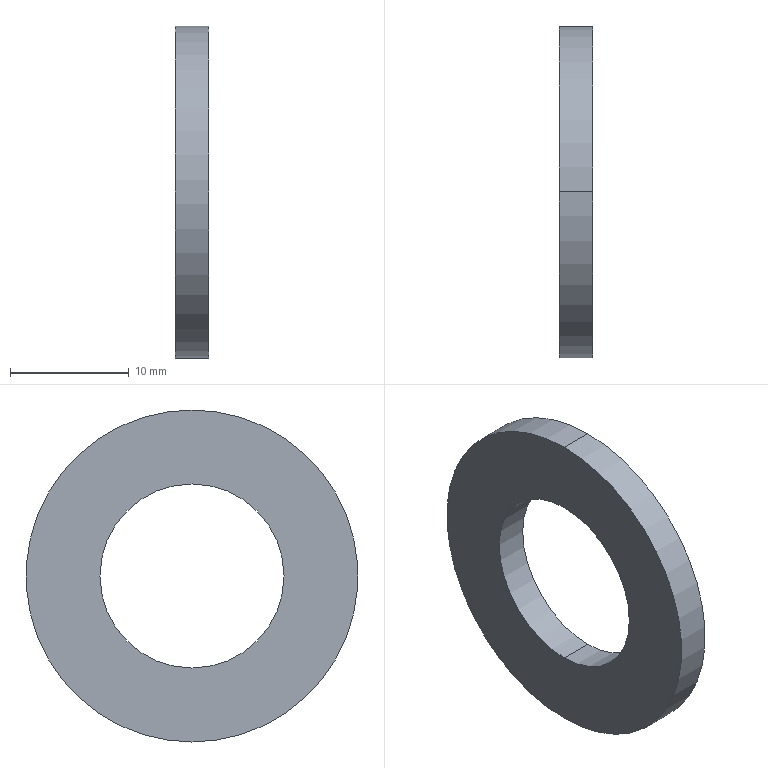Part | STEP file | flat washer narrow_am_B18.22M - Plain washer, 14 mm, narrow | 1 solid | 6 faces | box 2.8 x 28 x 28 mm | volume 1194 mm3 | cylinder 4 | plane 2 | commonest cylinder face diameters 15.52 x2 28 x2
STEP:
#1=CARTESIAN_POINT('',(0.,0.,0.));
#2=DIRECTION('',(0.,0.,1.));
#3=DIRECTION('',(1.,0.,0.));
#4=AXIS2_PLACEMENT_3D('',#1,#2,#3);
#5=CARTESIAN_POINT('',(0.,0.,14.));
#6=VERTEX_POINT('',#5);
#7=CARTESIAN_POINT('',(0.,0.,-14.));
#8=VERTEX_POINT('',#7);
#9=CARTESIAN_POINT('',(0.,0.,0.));
#10=DIRECTION('',(-1.,0.,0.));
#11=DIRECTION('',(0.,0.,1.));
#12=AXIS2_PLACEMENT_3D('',#9,#10,#11);
#13=CIRCLE('',#12,14.);
#14=CARTESIAN_POINT('',(-34.925,0.,0.));
#15=DIRECTION('',(-1.,0.,0.));
#16=DIRECTION('',(0.,0.,1.));
#17=AXIS2_PLACEMENT_3D('',#14,#15,#16);
#18=CYLINDRICAL_SURFACE('',#17,14.);
#19=CARTESIAN_POINT('',(0.,-34.925));
#20=DIRECTION('',(1.,0.));
#21=VECTOR('',#20,1.);
#22=LINE('',#19,#21);
#23=(GEOMETRIC_REPRESENTATION_CONTEXT(2)PARAMETRIC_REPRESENTATION_CONTEXT()REPRESENTATION_CONTEXT('',''));
#24=DEFINITIONAL_REPRESENTATION('',(#22),#23);
#25=PCURVE('',#18,#24);
#26=CARTESIAN_POINT('',(0.,7.76,0.));
#27=DIRECTION('',(-1.,0.,0.));
#28=DIRECTION('',(0.,0.,1.));
#29=AXIS2_PLACEMENT_3D('',#26,#27,#28);
#30=PLANE('',#29);
#31=CARTESIAN_POINT('',(0.,-7.76));
#32=DIRECTION('',(1.,0.));
#33=AXIS2_PLACEMENT_2D('',#31,#32);
#34=CIRCLE('',#33,14.);
#35=(GEOMETRIC_REPRESENTATION_CONTEXT(2)PARAMETRIC_REPRESENTATION_CONTEXT()REPRESENTATION_CONTEXT('',''));
#36=DEFINITIONAL_REPRESENTATION('',(#34),#35);
#37=PCURVE('',#30,#36);
#38=SURFACE_CURVE('',#13,(#25,#37),.PCURVE_S1.);
#39=EDGE_CURVE('',#6,#8,#38,.T.);
#40=ORIENTED_EDGE('',*,*,#39,.T.);
#41=CARTESIAN_POINT('',(-2.8,0.,-14.));
#42=VERTEX_POINT('',#41);
#43=CARTESIAN_POINT('',(-34.925,0.,-14.));
#44=DIRECTION('',(-1.,0.,0.));
#45=VECTOR('',#44,1.);
#46=LINE('',#43,#45);
#47=CARTESIAN_POINT('',(3.142,0.));
#48=DIRECTION('',(0.,1.));
#49=VECTOR('',#48,1.);
#50=LINE('',#47,#49);
#51=(GEOMETRIC_REPRESENTATION_CONTEXT(2)PARAMETRIC_REPRESENTATION_CONTEXT()REPRESENTATION_CONTEXT('',''));
#52=DEFINITIONAL_REPRESENTATION('',(#50),#51);
#53=PCURVE('',#18,#52);
#54=CARTESIAN_POINT('',(-34.925,0.,0.));
#55=DIRECTION('',(-1.,0.,0.));
#56=DIRECTION('',(0.,0.,1.));
#57=AXIS2_PLACEMENT_3D('',#54,#55,#56);
#58=CYLINDRICAL_SURFACE('',#57,14.);
#59=CARTESIAN_POINT('',(3.142,0.));
#60=DIRECTION('',(0.,1.));
#61=VECTOR('',#60,1.);
#62=LINE('',#59,#61);
#63=(GEOMETRIC_REPRESENTATION_CONTEXT(2)PARAMETRIC_REPRESENTATION_CONTEXT()REPRESENTATION_CONTEXT('',''));
#64=DEFINITIONAL_REPRESENTATION('',(#62),#63);
#65=PCURVE('',#58,#64);
#66=SURFACE_CURVE('',#46,(#53,#65),.PCURVE_S1.);
#67=EDGE_CURVE('',#8,#42,#66,.T.);
#68=ORIENTED_EDGE('',*,*,#67,.T.);
#69=CARTESIAN_POINT('',(-2.8,0.,14.));
#70=VERTEX_POINT('',#69);
#71=CARTESIAN_POINT('',(-2.8,0.,0.));
#72=DIRECTION('',(-1.,0.,0.));
#73=DIRECTION('',(0.,0.,1.));
#74=AXIS2_PLACEMENT_3D('',#71,#72,#73);
#75=CIRCLE('',#74,14.);
#76=CARTESIAN_POINT('',(0.,-32.125));
#77=DIRECTION('',(1.,0.));
#78=VECTOR('',#77,1.);
#79=LINE('',#76,#78);
#80=(GEOMETRIC_REPRESENTATION_CONTEXT(2)PARAMETRIC_REPRESENTATION_CONTEXT()REPRESENTATION_CONTEXT('',''));
#81=DEFINITIONAL_REPRESENTATION('',(#79),#80);
#82=PCURVE('',#18,#81);
#83=CARTESIAN_POINT('',(-2.8,14.,0.));
#84=DIRECTION('',(1.,0.,0.));
#85=DIRECTION('',(0.,0.,-1.));
#86=AXIS2_PLACEMENT_3D('',#83,#84,#85);
#87=PLANE('',#86);
#88=CARTESIAN_POINT('',(-14.,-14.));
#89=CARTESIAN_POINT('',(-14.,10.249));
#90=CARTESIAN_POINT('',(7.,-1.876));
#91=CARTESIAN_POINT('',(28.,-14.));
#92=CARTESIAN_POINT('',(7.,-26.124));
#93=CARTESIAN_POINT('',(-14.,-38.249));
#94=CARTESIAN_POINT('',(-14.,-14.));
#95=(BOUNDED_CURVE()B_SPLINE_CURVE(2,(#88,#89,#90,#91,#92,#93,#94),.UNSPECIFIED.,.T.,.F.)B_SPLINE_CURVE_WITH_KNOTS((1,2,2,2,2,1),(-2.094,0.,2.094,4.189,6.283,8.378),.UNSPECIFIED.)CURVE()GEOMETRIC_REPRESENTATION_ITEM()RATIONAL_B_SPLINE_CURVE((1.,0.5,1.,0.5,1.,0.5,1.))REPRESENTATION_ITEM(''));
#96=(GEOMETRIC_REPRESENTATION_CONTEXT(2)PARAMETRIC_REPRESENTATION_CONTEXT()REPRESENTATION_CONTEXT('',''));
#97=DEFINITIONAL_REPRESENTATION('',(#95),#96);
#98=PCURVE('',#87,#97);
#99=SURFACE_CURVE('',#75,(#82,#98),.PCURVE_S1.);
#100=EDGE_CURVE('',#70,#42,#99,.T.);
#101=ORIENTED_EDGE('',*,*,#100,.F.);
#102=CARTESIAN_POINT('',(-34.925,0.,14.));
#103=DIRECTION('',(-1.,0.,0.));
#104=VECTOR('',#103,1.);
#105=LINE('',#102,#104);
#106=CARTESIAN_POINT('',(0.,0.));
#107=DIRECTION('',(0.,1.));
#108=VECTOR('',#107,1.);
#109=LINE('',#106,#108);
#110=(GEOMETRIC_REPRESENTATION_CONTEXT(2)PARAMETRIC_REPRESENTATION_CONTEXT()REPRESENTATION_CONTEXT('',''));
#111=DEFINITIONAL_REPRESENTATION('',(#109),#110);
#112=PCURVE('',#18,#111);
#113=CARTESIAN_POINT('',(6.283,0.));
#114=DIRECTION('',(0.,1.));
#115=VECTOR('',#114,1.);
#116=LINE('',#113,#115);
#117=(GEOMETRIC_REPRESENTATION_CONTEXT(2)PARAMETRIC_REPRESENTATION_CONTEXT()REPRESENTATION_CONTEXT('',''));
#118=DEFINITIONAL_REPRESENTATION('',(#116),#117);
#119=PCURVE('',#58,#118);
#120=SURFACE_CURVE('',#105,(#112,#119),.PCURVE_S1.);
#121=EDGE_CURVE('',#6,#70,#120,.T.);
#122=ORIENTED_EDGE('',*,*,#121,.F.);
#123=EDGE_LOOP('',(#40,#68,#101,#122));
#124=FACE_BOUND('',#123,.T.);
#125=ADVANCED_FACE('',(#124),#18,.T.);
#126=CARTESIAN_POINT('',(0.,0.,7.76));
#127=VERTEX_POINT('',#126);
#128=CARTESIAN_POINT('',(-2.8,0.,7.76));
#129=VERTEX_POINT('',#128);
#130=CARTESIAN_POINT('',(-34.925,0.,7.76));
#131=DIRECTION('',(-1.,0.,0.));
#132=VECTOR('',#131,1.);
#133=LINE('',#130,#132);
#134=CARTESIAN_POINT('',(-34.925,0.,0.));
#135=DIRECTION('',(-1.,0.,0.));
#136=DIRECTION('',(0.,0.,1.));
#137=AXIS2_PLACEMENT_3D('',#134,#135,#136);
#138=CYLINDRICAL_SURFACE('',#137,7.76);
#139=CARTESIAN_POINT('',(6.283,0.));
#140=DIRECTION('',(0.,1.));
#141=VECTOR('',#140,1.);
#142=LINE('',#139,#141);
#143=(GEOMETRIC_REPRESENTATION_CONTEXT(2)PARAMETRIC_REPRESENTATION_CONTEXT()REPRESENTATION_CONTEXT('',''));
#144=DEFINITIONAL_REPRESENTATION('',(#142),#143);
#145=PCURVE('',#138,#144);
#146=CARTESIAN_POINT('',(-34.925,0.,0.));
#147=DIRECTION('',(-1.,0.,0.));
#148=DIRECTION('',(0.,0.,1.));
#149=AXIS2_PLACEMENT_3D('',#146,#147,#148);
#150=CYLINDRICAL_SURFACE('',#149,7.76);
#151=CARTESIAN_POINT('',(0.,0.));
#152=DIRECTION('',(0.,1.));
#153=VECTOR('',#152,1.);
#154=LINE('',#151,#153);
#155=(GEOMETRIC_REPRESENTATION_CONTEXT(2)PARAMETRIC_REPRESENTATION_CONTEXT()REPRESENTATION_CONTEXT('',''));
#156=DEFINITIONAL_REPRESENTATION('',(#154),#155);
#157=PCURVE('',#150,#156);
#158=SURFACE_CURVE('',#133,(#145,#157),.PCURVE_S1.);
#159=EDGE_CURVE('',#127,#129,#158,.T.);
#160=ORIENTED_EDGE('',*,*,#159,.T.);
#161=CARTESIAN_POINT('',(-2.8,0.,-7.76));
#162=VERTEX_POINT('',#161);
#163=CARTESIAN_POINT('',(-2.8,0.,0.));
#164=DIRECTION('',(-1.,0.,0.));
#165=DIRECTION('',(0.,0.,1.));
#166=AXIS2_PLACEMENT_3D('',#163,#164,#165);
#167=CIRCLE('',#166,7.76);
#168=CARTESIAN_POINT('',(0.,-32.125));
#169=DIRECTION('',(1.,0.));
#170=VECTOR('',#169,1.);
#171=LINE('',#168,#170);
#172=(GEOMETRIC_REPRESENTATION_CONTEXT(2)PARAMETRIC_REPRESENTATION_CONTEXT()REPRESENTATION_CONTEXT('',''));
#173=DEFINITIONAL_REPRESENTATION('',(#171),#172);
#174=PCURVE('',#138,#173);
#175=CARTESIAN_POINT('',(-7.76,-14.));
#176=CARTESIAN_POINT('',(-7.76,-0.5593));
#177=CARTESIAN_POINT('',(3.88,-7.28));
#178=CARTESIAN_POINT('',(15.52,-14.));
#179=CARTESIAN_POINT('',(3.88,-20.72));
#180=CARTESIAN_POINT('',(-7.76,-27.441));
#181=CARTESIAN_POINT('',(-7.76,-14.));
#182=(BOUNDED_CURVE()B_SPLINE_CURVE(2,(#175,#176,#177,#178,#179,#180,#181),.UNSPECIFIED.,.T.,.F.)B_SPLINE_CURVE_WITH_KNOTS((1,2,2,2,2,1),(-2.094,0.,2.094,4.189,6.283,8.378),.UNSPECIFIED.)CURVE()GEOMETRIC_REPRESENTATION_ITEM()RATIONAL_B_SPLINE_CURVE((1.,0.5,1.,0.5,1.,0.5,1.))REPRESENTATION_ITEM(''));
#183=(GEOMETRIC_REPRESENTATION_CONTEXT(2)PARAMETRIC_REPRESENTATION_CONTEXT()REPRESENTATION_CONTEXT('',''));
#184=DEFINITIONAL_REPRESENTATION('',(#182),#183);
#185=PCURVE('',#87,#184);
#186=SURFACE_CURVE('',#167,(#174,#185),.PCURVE_S1.);
#187=EDGE_CURVE('',#162,#129,#186,.T.);
#188=ORIENTED_EDGE('',*,*,#187,.F.);
#189=CARTESIAN_POINT('',(0.,0.,-7.76));
#190=VERTEX_POINT('',#189);
#191=CARTESIAN_POINT('',(-34.925,0.,-7.76));
#192=DIRECTION('',(-1.,0.,0.));
#193=VECTOR('',#192,1.);
#194=LINE('',#191,#193);
#195=CARTESIAN_POINT('',(3.142,0.));
#196=DIRECTION('',(0.,1.));
#197=VECTOR('',#196,1.);
#198=LINE('',#195,#197);
#199=(GEOMETRIC_REPRESENTATION_CONTEXT(2)PARAMETRIC_REPRESENTATION_CONTEXT()REPRESENTATION_CONTEXT('',''));
#200=DEFINITIONAL_REPRESENTATION('',(#198),#199);
#201=PCURVE('',#138,#200);
#202=CARTESIAN_POINT('',(3.142,0.));
#203=DIRECTION('',(0.,1.));
#204=VECTOR('',#203,1.);
#205=LINE('',#202,#204);
#206=(GEOMETRIC_REPRESENTATION_CONTEXT(2)PARAMETRIC_REPRESENTATION_CONTEXT()REPRESENTATION_CONTEXT('',''));
#207=DEFINITIONAL_REPRESENTATION('',(#205),#206);
#208=PCURVE('',#150,#207);
#209=SURFACE_CURVE('',#194,(#201,#208),.PCURVE_S1.);
#210=EDGE_CURVE('',#190,#162,#209,.T.);
#211=ORIENTED_EDGE('',*,*,#210,.F.);
#212=CARTESIAN_POINT('',(0.,0.,0.));
#213=DIRECTION('',(-1.,0.,0.));
#214=DIRECTION('',(0.,0.,1.));
#215=AXIS2_PLACEMENT_3D('',#212,#213,#214);
#216=CIRCLE('',#215,7.76);
#217=CARTESIAN_POINT('',(0.,-34.925));
#218=DIRECTION('',(1.,0.));
#219=VECTOR('',#218,1.);
#220=LINE('',#217,#219);
#221=(GEOMETRIC_REPRESENTATION_CONTEXT(2)PARAMETRIC_REPRESENTATION_CONTEXT()REPRESENTATION_CONTEXT('',''));
#222=DEFINITIONAL_REPRESENTATION('',(#220),#221);
#223=PCURVE('',#138,#222);
#224=CARTESIAN_POINT('',(0.,-7.76));
#225=DIRECTION('',(1.,0.));
#226=AXIS2_PLACEMENT_2D('',#224,#225);
#227=CIRCLE('',#226,7.76);
#228=(GEOMETRIC_REPRESENTATION_CONTEXT(2)PARAMETRIC_REPRESENTATION_CONTEXT()REPRESENTATION_CONTEXT('',''));
#229=DEFINITIONAL_REPRESENTATION('',(#227),#228);
#230=PCURVE('',#30,#229);
#231=SURFACE_CURVE('',#216,(#223,#230),.PCURVE_S1.);
#232=EDGE_CURVE('',#190,#127,#231,.T.);
#233=ORIENTED_EDGE('',*,*,#232,.T.);
#234=EDGE_LOOP('',(#160,#188,#211,#233));
#235=FACE_BOUND('',#234,.F.);
#236=ADVANCED_FACE('',(#235),#138,.F.);
#237=CARTESIAN_POINT('',(-2.8,0.,0.));
#238=DIRECTION('',(-1.,0.,0.));
#239=DIRECTION('',(0.,0.,1.));
#240=AXIS2_PLACEMENT_3D('',#237,#238,#239);
#241=CIRCLE('',#240,7.76);
#242=CARTESIAN_POINT('',(0.,-32.125));
#243=DIRECTION('',(1.,0.));
#244=VECTOR('',#243,1.);
#245=LINE('',#242,#244);
#246=(GEOMETRIC_REPRESENTATION_CONTEXT(2)PARAMETRIC_REPRESENTATION_CONTEXT()REPRESENTATION_CONTEXT('',''));
#247=DEFINITIONAL_REPRESENTATION('',(#245),#246);
#248=PCURVE('',#150,#247);
#249=CARTESIAN_POINT('',(-7.76,-14.));
#250=CARTESIAN_POINT('',(-7.76,-0.5593));
#251=CARTESIAN_POINT('',(3.88,-7.28));
#252=CARTESIAN_POINT('',(15.52,-14.));
#253=CARTESIAN_POINT('',(3.88,-20.72));
#254=CARTESIAN_POINT('',(-7.76,-27.441));
#255=CARTESIAN_POINT('',(-7.76,-14.));
#256=(BOUNDED_CURVE()B_SPLINE_CURVE(2,(#249,#250,#251,#252,#253,#254,#255),.UNSPECIFIED.,.T.,.F.)B_SPLINE_CURVE_WITH_KNOTS((1,2,2,2,2,1),(-2.094,0.,2.094,4.189,6.283,8.378),.UNSPECIFIED.)CURVE()GEOMETRIC_REPRESENTATION_ITEM()RATIONAL_B_SPLINE_CURVE((1.,0.5,1.,0.5,1.,0.5,1.))REPRESENTATION_ITEM(''));
#257=(GEOMETRIC_REPRESENTATION_CONTEXT(2)PARAMETRIC_REPRESENTATION_CONTEXT()REPRESENTATION_CONTEXT('',''));
#258=DEFINITIONAL_REPRESENTATION('',(#256),#257);
#259=PCURVE('',#87,#258);
#260=SURFACE_CURVE('',#241,(#248,#259),.PCURVE_S1.);
#261=EDGE_CURVE('',#129,#162,#260,.T.);
#262=ORIENTED_EDGE('',*,*,#261,.F.);
#263=ORIENTED_EDGE('',*,*,#159,.F.);
#264=CARTESIAN_POINT('',(0.,0.,0.));
#265=DIRECTION('',(-1.,0.,0.));
#266=DIRECTION('',(0.,0.,1.));
#267=AXIS2_PLACEMENT_3D('',#264,#265,#266);
#268=CIRCLE('',#267,7.76);
#269=CARTESIAN_POINT('',(0.,-34.925));
#270=DIRECTION('',(1.,0.));
#271=VECTOR('',#270,1.);
#272=LINE('',#269,#271);
#273=(GEOMETRIC_REPRESENTATION_CONTEXT(2)PARAMETRIC_REPRESENTATION_CONTEXT()REPRESENTATION_CONTEXT('',''));
#274=DEFINITIONAL_REPRESENTATION('',(#272),#273);
#275=PCURVE('',#150,#274);
#276=CARTESIAN_POINT('',(0.,-7.76));
#277=DIRECTION('',(1.,0.));
#278=AXIS2_PLACEMENT_2D('',#276,#277);
#279=CIRCLE('',#278,7.76);
#280=(GEOMETRIC_REPRESENTATION_CONTEXT(2)PARAMETRIC_REPRESENTATION_CONTEXT()REPRESENTATION_CONTEXT('',''));
#281=DEFINITIONAL_REPRESENTATION('',(#279),#280);
#282=PCURVE('',#30,#281);
#283=SURFACE_CURVE('',#268,(#275,#282),.PCURVE_S1.);
#284=EDGE_CURVE('',#127,#190,#283,.T.);
#285=ORIENTED_EDGE('',*,*,#284,.T.);
#286=ORIENTED_EDGE('',*,*,#210,.T.);
#287=EDGE_LOOP('',(#262,#263,#285,#286));
#288=FACE_BOUND('',#287,.F.);
#289=ADVANCED_FACE('',(#288),#150,.F.);
#290=ORIENTED_EDGE('',*,*,#39,.F.);
#291=CARTESIAN_POINT('',(0.,0.,0.));
#292=DIRECTION('',(-1.,0.,0.));
#293=DIRECTION('',(0.,0.,1.));
#294=AXIS2_PLACEMENT_3D('',#291,#292,#293);
#295=CIRCLE('',#294,14.);
#296=CARTESIAN_POINT('',(0.,-7.76));
#297=DIRECTION('',(1.,0.));
#298=AXIS2_PLACEMENT_2D('',#296,#297);
#299=CIRCLE('',#298,14.);
#300=(GEOMETRIC_REPRESENTATION_CONTEXT(2)PARAMETRIC_REPRESENTATION_CONTEXT()REPRESENTATION_CONTEXT('',''));
#301=DEFINITIONAL_REPRESENTATION('',(#299),#300);
#302=PCURVE('',#30,#301);
#303=CARTESIAN_POINT('',(0.,-34.925));
#304=DIRECTION('',(1.,0.));
#305=VECTOR('',#304,1.);
#306=LINE('',#303,#305);
#307=(GEOMETRIC_REPRESENTATION_CONTEXT(2)PARAMETRIC_REPRESENTATION_CONTEXT()REPRESENTATION_CONTEXT('',''));
#308=DEFINITIONAL_REPRESENTATION('',(#306),#307);
#309=PCURVE('',#58,#308);
#310=SURFACE_CURVE('',#295,(#302,#309),.PCURVE_S1.);
#311=EDGE_CURVE('',#8,#6,#310,.T.);
#312=ORIENTED_EDGE('',*,*,#311,.F.);
#313=EDGE_LOOP('',(#290,#312));
#314=FACE_BOUND('',#313,.T.);
#315=ORIENTED_EDGE('',*,*,#284,.T.);
#316=ORIENTED_EDGE('',*,*,#232,.T.);
#317=EDGE_LOOP('',(#315,#316));
#318=FACE_BOUND('',#317,.T.);
#319=ADVANCED_FACE('',(#314,#318),#30,.F.);
#320=ORIENTED_EDGE('',*,*,#67,.F.);
#321=ORIENTED_EDGE('',*,*,#311,.T.);
#322=ORIENTED_EDGE('',*,*,#121,.T.);
#323=CARTESIAN_POINT('',(-2.8,0.,0.));
#324=DIRECTION('',(-1.,0.,0.));
#325=DIRECTION('',(0.,0.,1.));
#326=AXIS2_PLACEMENT_3D('',#323,#324,#325);
#327=CIRCLE('',#326,14.);
#328=CARTESIAN_POINT('',(0.,-32.125));
#329=DIRECTION('',(1.,0.));
#330=VECTOR('',#329,1.);
#331=LINE('',#328,#330);
#332=(GEOMETRIC_REPRESENTATION_CONTEXT(2)PARAMETRIC_REPRESENTATION_CONTEXT()REPRESENTATION_CONTEXT('',''));
#333=DEFINITIONAL_REPRESENTATION('',(#331),#332);
#334=PCURVE('',#58,#333);
#335=CARTESIAN_POINT('',(-14.,-14.));
#336=CARTESIAN_POINT('',(-14.,10.249));
#337=CARTESIAN_POINT('',(7.,-1.876));
#338=CARTESIAN_POINT('',(28.,-14.));
#339=CARTESIAN_POINT('',(7.,-26.124));
#340=CARTESIAN_POINT('',(-14.,-38.249));
#341=CARTESIAN_POINT('',(-14.,-14.));
#342=(BOUNDED_CURVE()B_SPLINE_CURVE(2,(#335,#336,#337,#338,#339,#340,#341),.UNSPECIFIED.,.T.,.F.)B_SPLINE_CURVE_WITH_KNOTS((1,2,2,2,2,1),(-2.094,0.,2.094,4.189,6.283,8.378),.UNSPECIFIED.)CURVE()GEOMETRIC_REPRESENTATION_ITEM()RATIONAL_B_SPLINE_CURVE((1.,0.5,1.,0.5,1.,0.5,1.))REPRESENTATION_ITEM(''));
#343=(GEOMETRIC_REPRESENTATION_CONTEXT(2)PARAMETRIC_REPRESENTATION_CONTEXT()REPRESENTATION_CONTEXT('',''));
#344=DEFINITIONAL_REPRESENTATION('',(#342),#343);
#345=PCURVE('',#87,#344);
#346=SURFACE_CURVE('',#327,(#334,#345),.PCURVE_S1.);
#347=EDGE_CURVE('',#42,#70,#346,.T.);
#348=ORIENTED_EDGE('',*,*,#347,.F.);
#349=EDGE_LOOP('',(#320,#321,#322,#348));
#350=FACE_BOUND('',#349,.T.);
#351=ADVANCED_FACE('',(#350),#58,.T.);
#352=ORIENTED_EDGE('',*,*,#261,.F.);
#353=ORIENTED_EDGE('',*,*,#187,.F.);
#354=EDGE_LOOP('',(#352,#353));
#355=FACE_BOUND('',#354,.T.);
#356=ORIENTED_EDGE('',*,*,#100,.T.);
#357=ORIENTED_EDGE('',*,*,#347,.T.);
#358=EDGE_LOOP('',(#356,#357));
#359=FACE_BOUND('',#358,.T.);
#360=ADVANCED_FACE('',(#355,#359),#87,.F.);
#361=CLOSED_SHELL('',(#125,#236,#289,#319,#351,#360));
#362=MANIFOLD_SOLID_BREP('',#361);
#363=(LENGTH_UNIT()NAMED_UNIT(*)SI_UNIT(.MILLI.,.METRE.));
#364=UNCERTAINTY_MEASURE_WITH_UNIT(LENGTH_MEASURE(0.0000001),#363,'','');
#365=(NAMED_UNIT(*)PLANE_ANGLE_UNIT()SI_UNIT($,.RADIAN.));
#366=(NAMED_UNIT(*)SI_UNIT($,.STERADIAN.)SOLID_ANGLE_UNIT());
#367=(GEOMETRIC_REPRESENTATION_CONTEXT(3)GLOBAL_UNCERTAINTY_ASSIGNED_CONTEXT((#364))GLOBAL_UNIT_ASSIGNED_CONTEXT((#363,#365,#366))REPRESENTATION_CONTEXT('',''));
#368=ADVANCED_BREP_SHAPE_REPRESENTATION('',(#4,#362),#367);